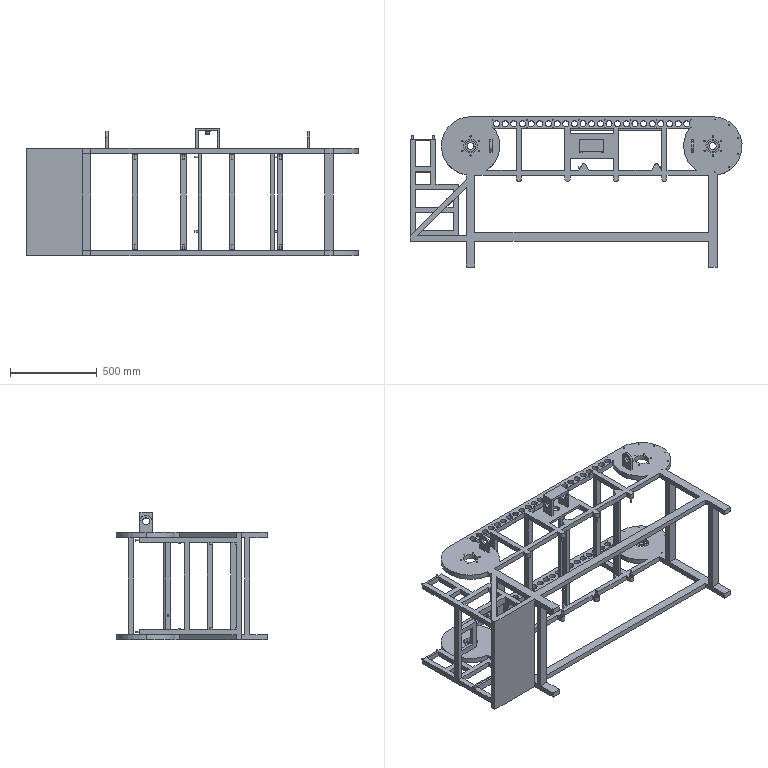Part | SolidWorks | features BaseBody 1 | 1 solid | 646 faces | box 1919 x 868.884 x 736.414 mm | volume 43603869 mm3 | cylinder 348 | plane 264 | cone 34 | commonest cylinder face diameters 35 x92 4 x64 8 x56 10 x36 5 x24 20 x22